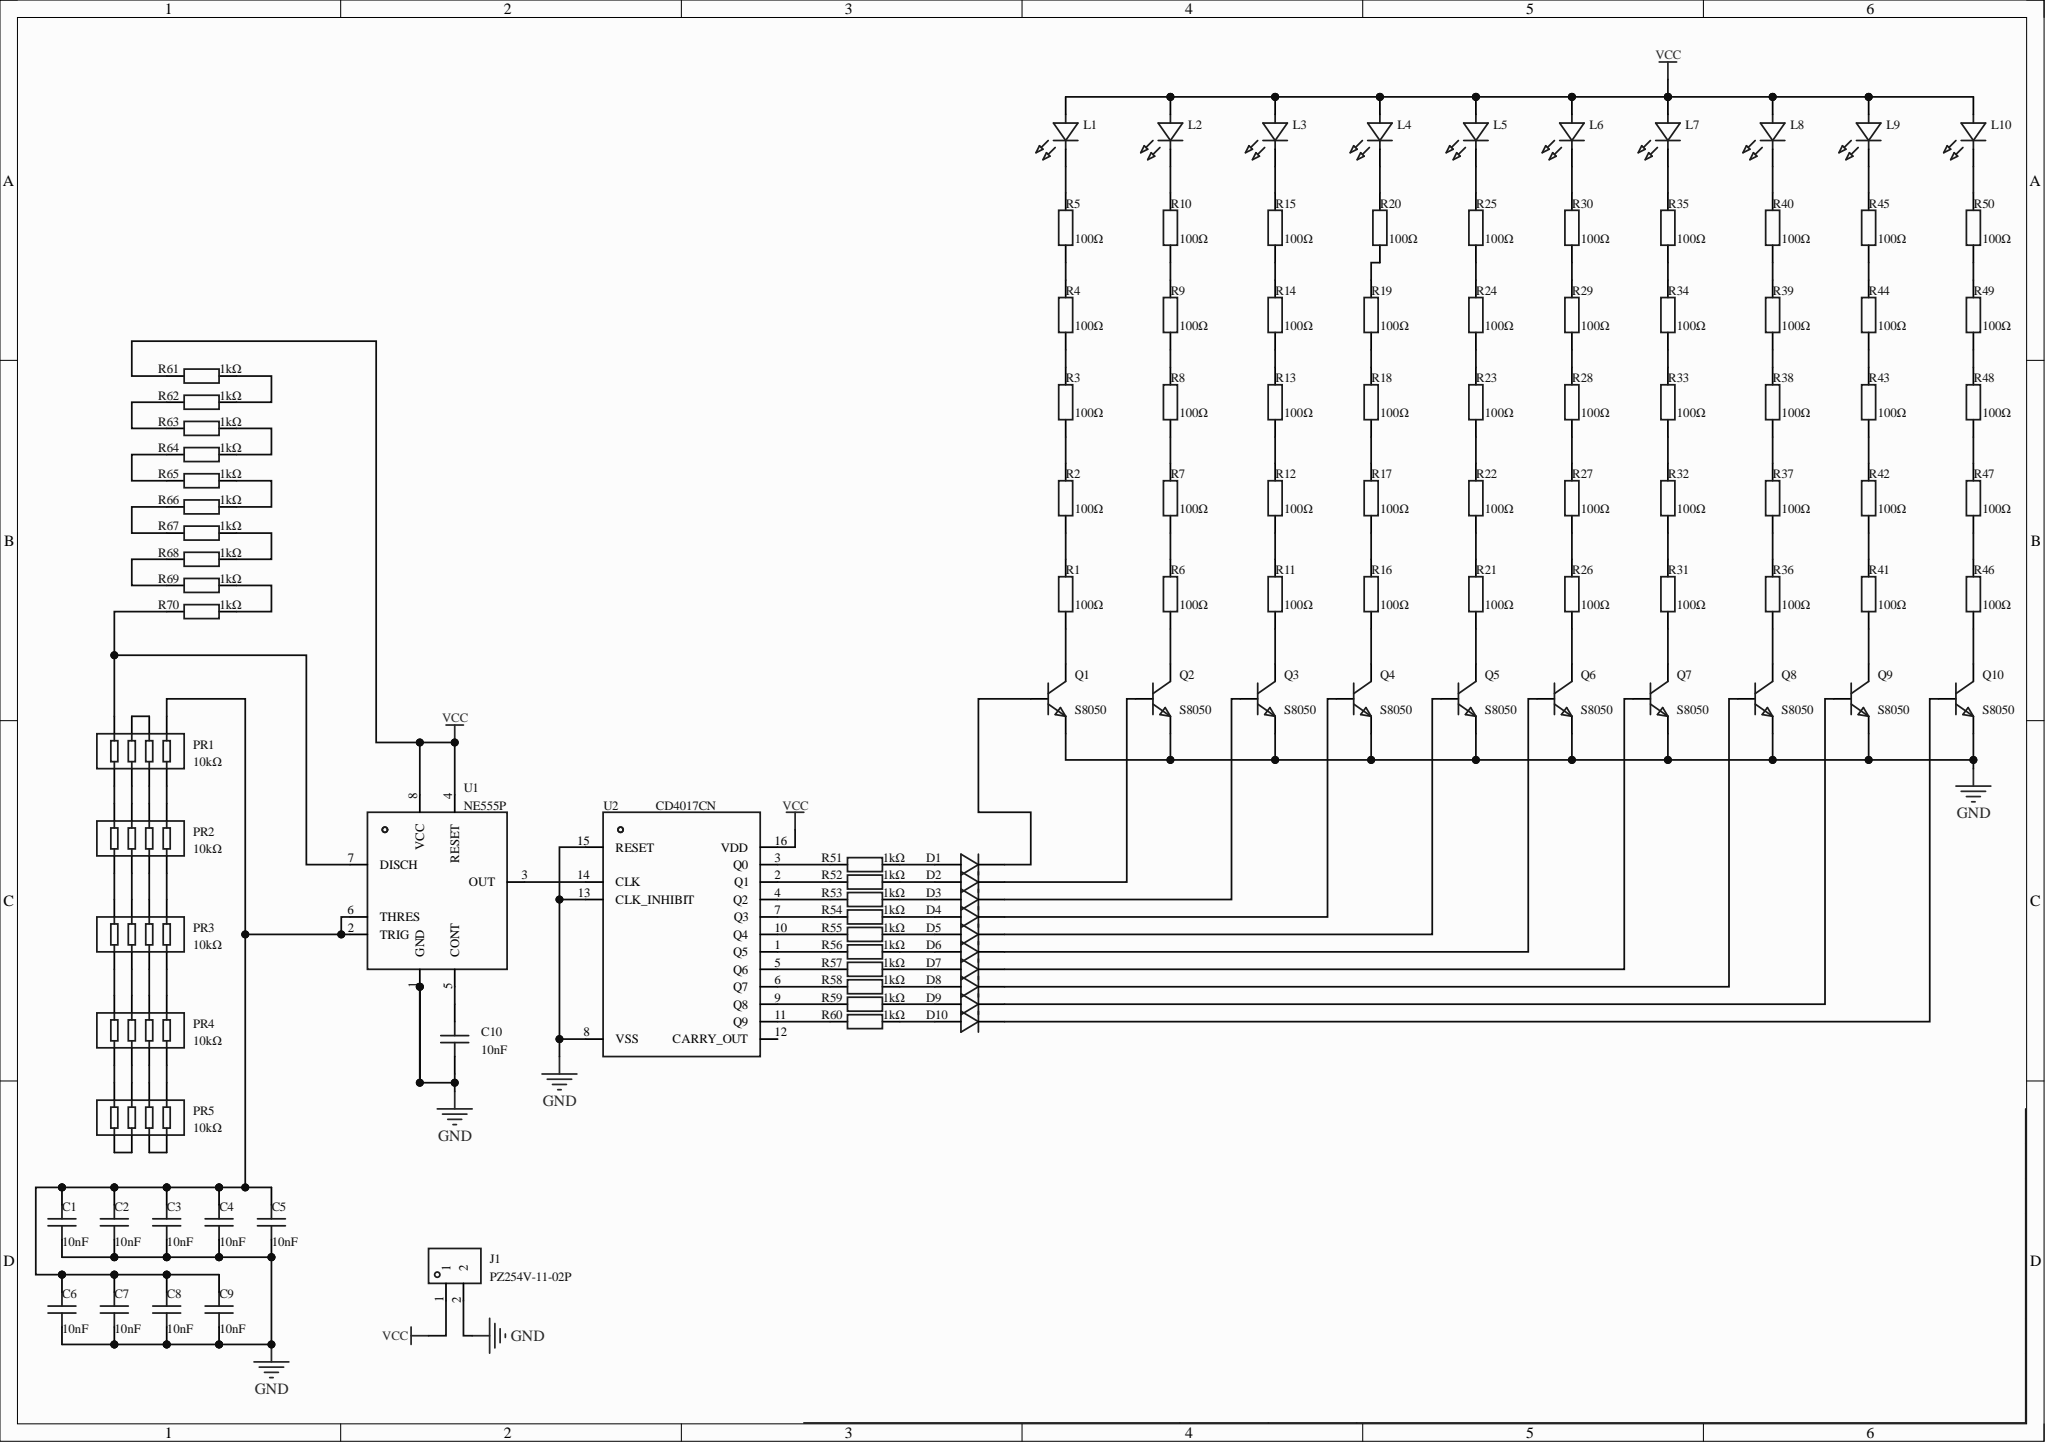Circuit board | Altium Designer | 118 parts | 124 nets
Bill of materials:
Comment,Description,Designator,Footprint,LibRef,Quantity
"10nF","容值:10nF;精度:±20%;额定电压:1kV;温度系数:Y5V;","C1, C2, C3, C4, C5, C6, C7, C8, C9, C10","CAP-TH_L8.0-W2.8-P5.08-D0.6","CC3A103MC1IEF48C30MF","10"
"1N4148TR","二极管配置:-;正向压降(Vf):1V@10mA;直流反向耐压(Vr):100V;整流电流:200mA;反向恢复时间(Trr):4ns;","D1, D2, D3, D4, D5, D6, D7, D8, D9, D10","DO-35_BD2.0-L4.2-P8.20-D0.5-RD","1N4148TR_C84410","10"
"PZ254V-11-02P","插针结构:1x2P;间距:2.54mm;行距:-;圆针/方针:方针;安装方式:直插;排数:单排;总PIN位数:2P;额定电流:3A;额定电压:250V;配合针长度:6mm;塑高:2.5mm;端接针长度:3mm;触头材质:黄铜;触头镀层:-;工作温度:-40℃~+105℃;颜色:黑色;","J1","HDR-TH_2P-P2.54-V-M","PZ254V-11-02P","1"
"XL-502SURD","灯头类型:5mm圆形灯头;发光颜色:红色;正向压降(Vf):2.4V;功率:70mW;正向电流:20mA;波长:615nm~625nm;二极管配置:-;透镜颜色:红色透镜;色温:-;发光强度:300mcd;发光角度:35°;载带方式:-;工作温度:-25℃~+85℃;","L1, L2, L3, L4, L5, L6, L7, L8, L9, L10","LED-TH_BD5.9-P2.54-RD_RED","XL-502SURD","10"
"10kΩ","","PR1, PR2, PR3, PR4, PR5","RES-ARRAY-TH_8P-L20.3-W2.5-P2.54","4608X-102-103LF","5"
"S8050","晶体管类型:NPN;集电极电流(Ic):500mA;集射极击穿电压(Vceo):25V;耗散功率(Pd):625mW;直流电流增益(hFE):160@50mA,1V;","Q1, Q2, Q3, Q4, Q5, Q6, Q7, Q8, Q9, Q10","TO-92-3_L4.5-W3.5-P1.27-L","S8050_C2931492","10"
"100Ω","","R1, R2, R3, R4, R5, R6, R7, R8, R9, R10, R11, R12, R13, R14, R15, R16, R17, R18, R19, R20, R21, R22, R23, R24, R25, R26, R27, R28, R29, R30, R31, R32, R33, R34, R35, R36, R37, R38, R39, R40, R41, R42, R43, R44, R45, R46, R47, R48, R49, R50","RES-TH_BD2.2-L6.5-P10.50-D0.6","MFR0W4F1000A50","50"
"1kΩ","","R51, R52, R53, R54, R55, R56, R57, R58, R59, R60, R61, R62, R63, R64, R65, R66, R67, R68, R69, R70","RES-TH_BD2.5-L6.5-P10.50-D0.6","MFR0W4F1001A50","20"
"NE555P","这些器件是精密定时电路，能够产生精确的时间延迟或振荡。在延时或单稳态工作模式下，定时时间间隔由单个外部电阻和电容网络控制。在无稳态工作模式下，频率和占空比可通过两个外部电阻和一个外部电容分别控制","U1","DIP-8_L9.8-W6.6-P2.54-LS7.6-BL","NE555P","1"
"CD4017CN","CD4017BE升级替代料，建议试样，5 阶 Johnson 译码计数器","U2","PDIP-16_L19.3-W6.4-P2.54-LS7.94-BL","CD4017CN","1"
Netlist (Protel format):
[
C1
CAP-TH_L8.0-W2.8-P5.08-D0.6
10nF



]
[
C2
CAP-TH_L8.0-W2.8-P5.08-D0.6
10nF



]
[
C3
CAP-TH_L8.0-W2.8-P5.08-D0.6
10nF



]
[
C4
CAP-TH_L8.0-W2.8-P5.08-D0.6
10nF



]
[
C5
CAP-TH_L8.0-W2.8-P5.08-D0.6
10nF



]
[
C6
CAP-TH_L8.0-W2.8-P5.08-D0.6
10nF



]
[
C7
CAP-TH_L8.0-W2.8-P5.08-D0.6
10nF



]
[
C8
CAP-TH_L8.0-W2.8-P5.08-D0.6
10nF



]
[
C9
CAP-TH_L8.0-W2.8-P5.08-D0.6
10nF



]
[
C10
CAP-TH_L8.0-W2.8-P5.08-D0.6
10nF



]
[
D1
DO-35_BD2.0-L4.2-P8.20-D0.5-RD
1N4148TR



]
[
D2
DO-35_BD2.0-L4.2-P8.20-D0.5-RD
1N4148TR



]
[
D3
DO-35_BD2.0-L4.2-P8.20-D0.5-RD
1N4148TR



]
[
D4
DO-35_BD2.0-L4.2-P8.20-D0.5-RD
1N4148TR



]
[
D5
DO-35_BD2.0-L4.2-P8.20-D0.5-RD
1N4148TR



]
[
D6
DO-35_BD2.0-L4.2-P8.20-D0.5-RD
1N4148TR



]
[
D7
DO-35_BD2.0-L4.2-P8.20-D0.5-RD
1N4148TR



]
[
D8
DO-35_BD2.0-L4.2-P8.20-D0.5-RD
1N4148TR



]
[
D9
DO-35_BD2.0-L4.2-P8.20-D0.5-RD
1N4148TR



]
[
D10
DO-35_BD2.0-L4.2-P8.20-D0.5-RD
1N4148TR



]
[
J1
HDR-TH_2P-P2.54-V-M
PZ254V-11-02P



]
[
L1
LED-TH_BD5.9-P2.54-RD_RED
XL-502SURD



]
[
L2
LED-TH_BD5.9-P2.54-RD_RED
XL-502SURD



]
[
L3
LED-TH_BD5.9-P2.54-RD_RED
XL-502SURD



]
[
L4
LED-TH_BD5.9-P2.54-RD_RED
XL-502SURD



]
[
L5
LED-TH_BD5.9-P2.54-RD_RED
XL-502SURD



]
[
L6
LED-TH_BD5.9-P2.54-RD_RED
XL-502SURD



]
[
L7
LED-TH_BD5.9-P2.54-RD_RED
XL-502SURD



]
[
L8
LED-TH_BD5.9-P2.54-RD_RED
XL-502SURD



]
[
L9
LED-TH_BD5.9-P2.54-RD_RED
XL-502SURD



]
[
L10
LED-TH_BD5.9-P2.54-RD_RED
XL-502SURD



]
[
PR1
RES-ARRAY-TH_8P-L20.3-W2.5-P2.54
10kΩ



]
[
PR2
RES-ARRAY-TH_8P-L20.3-W2.5-P2.54
10kΩ



]
[
PR3
RES-ARRAY-TH_8P-L20.3-W2.5-P2.54
10kΩ



]
[
PR4
RES-ARRAY-TH_8P-L20.3-W2.5-P2.54
10kΩ



]
[
PR5
RES-ARRAY-TH_8P-L20.3-W2.5-P2.54
10kΩ



]
[
Q1
TO-92-3_L4.5-W3.5-P1.27-L
S8050



]
[
Q2
TO-92-3_L4.5-W3.5-P1.27-L
S8050



]
[
Q3
TO-92-3_L4.5-W3.5-P1.27-L
S8050



]
[
Q4
TO-92-3_L4.5-W3.5-P1.27-L
S8050



]
[
Q5
TO-92-3_L4.5-W3.5-P1.27-L
S8050



]
[
Q6
TO-92-3_L4.5-W3.5-P1.27-L
S8050



]
[
Q7
TO-92-3_L4.5-W3.5-P1.27-L
S8050



]
[
Q8
TO-92-3_L4.5-W3.5-P1.27-L
S8050



]
[
Q9
TO-92-3_L4.5-W3.5-P1.27-L
S8050



]
[
Q10
TO-92-3_L4.5-W3.5-P1.27-L
S8050



]
[
R1
RES-TH_BD2.2-L6.5-P10.50-D0.6
100Ω



]
[
R2
RES-TH_BD2.2-L6.5-P10.50-D0.6
100Ω



]
[
R3
RES-TH_BD2.2-L6.5-P10.50-D0.6
100Ω



]
[
R4
RES-TH_BD2.2-L6.5-P10.50-D0.6
100Ω



]
[
R5
RES-TH_BD2.2-L6.5-P10.50-D0.6
100Ω



]
[
R6
RES-TH_BD2.2-L6.5-P10.50-D0.6
100Ω



]
[
R7
RES-TH_BD2.2-L6.5-P10.50-D0.6
100Ω



]
[
R8
RES-TH_BD2.2-L6.5-P10.50-D0.6
100Ω



]
[
R9
RES-TH_BD2.2-L6.5-P10.50-D0.6
100Ω



]
[
R10
RES-TH_BD2.2-L6.5-P10.50-D0.6
100Ω



]
[
R11
RES-TH_BD2.2-L6.5-P10.50-D0.6
100Ω



]
[
R12
RES-TH_BD2.2-L6.5-P10.50-D0.6
100Ω



]
[
R13
RES-TH_BD2.2-L6.5-P10.50-D0.6
100Ω



]
[
R14
RES-TH_BD2.2-L6.5-P10.50-D0.6
100Ω



]
[
R15
RES-TH_BD2.2-L6.5-P10.50-D0.6
100Ω



]
[
R16
RES-TH_BD2.2-L6.5-P10.50-D0.6
100Ω



]
[
R17
RES-TH_BD2.2-L6.5-P10.50-D0.6
100Ω



]
[
R18
RES-TH_BD2.2-L6.5-P10.50-D0.6
100Ω



]
[
R19
RES-TH_BD2.2-L6.5-P10.50-D0.6
100Ω



]
[
R20
RES-TH_BD2.2-L6.5-P10.50-D0.6
100Ω



]
[
R21
RES-TH_BD2.2-L6.5-P10.50-D0.6
100Ω



]
[
R22
RES-TH_BD2.2-L6.5-P10.50-D0.6
100Ω



]
[
R23
RES-TH_BD2.2-L6.5-P10.50-D0.6
100Ω



]
[
R24
RES-TH_BD2.2-L6.5-P10.50-D0.6
100Ω



]
[
R25
RES-TH_BD2.2-L6.5-P10.50-D0.6
100Ω



]
[
R26
RES-TH_BD2.2-L6.5-P10.50-D0.6
100Ω



]
[
R27
RES-TH_BD2.2-L6.5-P10.50-D0.6
100Ω



]
[
R28
RES-TH_BD2.2-L6.5-P10.50-D0.6
100Ω



]
[
R29
RES-TH_BD2.2-L6.5-P10.50-D0.6
100Ω



]
[
R30
RES-TH_BD2.2-L6.5-P10.50-D0.6
100Ω



]
[
R31
RES-TH_BD2.2-L6.5-P10.50-D0.6
100Ω



]
[
R32
RES-TH_BD2.2-L6.5-P10.50-D0.6
100Ω



]
[
R33
RES-TH_BD2.2-L6.5-P10.50-D0.6
100Ω



]
[
R34
RES-TH_BD2.2-L6.5-P10.50-D0.6
100Ω



]
[
R35
RES-TH_BD2.2-L6.5-P10.50-D0.6
100Ω



]
[
R36
RES-TH_BD2.2-L6.5-P10.50-D0.6
100Ω



]
[
R37
RES-TH_BD2.2-L6.5-P10.50-D0.6
100Ω



]
[
R38
RES-TH_BD2.2-L6.5-P10.50-D0.6
100Ω



]
[
R39
RES-TH_BD2.2-L6.5-P10.50-D0.6
100Ω



]
[
R40
RES-TH_BD2.2-L6.5-P10.50-D0.6
100Ω



]
[
R41
RES-TH_BD2.2-L6.5-P10.50-D0.6
100Ω



]
[
R42
RES-TH_BD2.2-L6.5-P10.50-D0.6
100Ω



]
[
R43
RES-TH_BD2.2-L6.5-P10.50-D0.6
100Ω



]
[
R44
RES-TH_BD2.2-L6.5-P10.50-D0.6
100Ω



]
[
R45
RES-TH_BD2.2-L6.5-P10.50-D0.6
100Ω



]
[
R46
RES-TH_BD2.2-L6.5-P10.50-D0.6
100Ω



]
[
R47
RES-TH_BD2.2-L6.5-P10.50-D0.6
100Ω



]
[
R48
RES-TH_BD2.2-L6.5-P10.50-D0.6
100Ω



]
[
R49
RES-TH_BD2.2-L6.5-P10.50-D0.6
100Ω



]
[
R50
RES-TH_BD2.2-L6.5-P10.50-D0.6
100Ω



]
[
R51
RES-TH_BD2.5-L6.5-P10.50-D0.6
1kΩ



]
[
R52
RES-TH_BD2.5-L6.5-P10.50-D0.6
1kΩ



]
[
R53
RES-TH_BD2.5-L6.5-P10.50-D0.6
1kΩ



]
[
R54
RES-TH_BD2.5-L6.5-P10.50-D0.6
1kΩ



]
[
R55
RES-TH_BD2.5-L6.5-P10.50-D0.6
1kΩ



]
[
R56
RES-TH_BD2.5-L6.5-P10.50-D0.6
1kΩ



]
[
R57
RES-TH_BD2.5-L6.5-P10.50-D0.6
1kΩ



]
[
R58
RES-TH_BD2.5-L6.5-P10.50-D0.6
1kΩ



]
[
R59
RES-TH_BD2.5-L6.5-P10.50-D0.6
1kΩ



]
[
R60
RES-TH_BD2.5-L6.5-P10.50-D0.6
1kΩ



]
[
R61
RES-TH_BD2.5-L6.5-P10.50-D0.6
1kΩ



]
[
R62
RES-TH_BD2.5-L6.5-P10.50-D0.6
1kΩ



]
[
R63
RES-TH_BD2.5-L6.5-P10.50-D0.6
1kΩ



]
[
R64
RES-TH_BD2.5-L6.5-P10.50-D0.6
1kΩ



]
[
R65
RES-TH_BD2.5-L6.5-P10.50-D0.6
1kΩ



]
[
R66
RES-TH_BD2.5-L6.5-P10.50-D0.6
1kΩ



]
[
R67
RES-TH_BD2.5-L6.5-P10.50-D0.6
1kΩ



]
[
R68
RES-TH_BD2.5-L6.5-P10.50-D0.6
1kΩ



]
[
R69
RES-TH_BD2.5-L6.5-P10.50-D0.6
1kΩ



]
[
R70
RES-TH_BD2.5-L6.5-P10.50-D0.6
1kΩ



]
[
U1
DIP-8_L9.8-W6.6-P2.54-LS7.6-BL
NE555P



]
[
U2
PDIP-16_L19.3-W6.4-P2.54-LS7.94-BL
CD4017CN



]
(
VCC
J1-1
L1-2
L2-2
L3-2
L4-2
L5-2
L6-2
L7-2
L8-2
L9-2
L10-2
R61-1
U1-4
U1-8
U2-16
)
(
NetU1_3
U1-3
U2-14
)
(
NetR69_2
R69-2
R70-2
)
(
NetR68_1
R68-1
R69-1
)
(
NetR67_2
R67-2
R68-2
)
(
NetR66_1
R66-1
R67-1
)
(
NetR65_2
R65-2
R66-2
)
(
NetR64_1
R64-1
R65-1
)
(
NetR63_2
R63-2
R64-2
)
(
NetR62_1
R62-1
R63-1
)
(
NetR61_2
R61-2
R62-2
)
(
NetR60_1
R60-1
U2-11
)
(
NetR59_1
R59-1
U2-9
)
(
NetR58_1
R58-1
U2-6
)
(
NetR57_1
R57-1
U2-5
)
(
NetR56_1
R56-1
U2-1
)
(
NetR55_1
R55-1
U2-10
)
(
NetR54_1
R54-1
U2-7
)
(
NetR53_1
R53-1
U2-4
)
(
NetR52_1
R52-1
U2-2
)
(
NetR51_1
R51-1
U2-3
)
(
NetR49_2
R49-2
R50-1
)
(
NetR48_2
R48-2
R49-1
)
(
NetR47_2
R47-2
R48-1
)
(
NetR46_2
R46-2
R47-1
)
(
NetR44_2
R44-2
R45-1
)
(
NetR43_2
R43-2
R44-1
)
(
NetR42_2
R42-2
R43-1
)
(
NetR41_2
R41-2
R42-1
)
(
NetR39_2
R39-2
R40-1
)
(
NetR38_2
R38-2
R39-1
)
(
NetR37_2
R37-2
R38-1
)
(
NetR36_2
R36-2
R37-1
)
(
NetR34_2
R34-2
R35-1
)
(
NetR33_2
R33-2
R34-1
)
(
NetR32_2
R32-2
R33-1
)
(
NetR31_2
R31-2
R32-1
)
(
NetR29_2
R29-2
R30-1
)
(
NetR28_2
R28-2
R29-1
)
(
NetR27_2
R27-2
R28-1
)
(
NetR26_2
R26-2
R27-1
)
(
NetR24_2
R24-2
R25-1
)
(
NetR23_2
R23-2
R24-1
)
(
NetR22_2
R22-2
R23-1
)
(
NetR21_2
R21-2
R22-1
)
(
NetR19_2
R19-2
R20-1
)
(
NetR18_2
R18-2
R19-1
)
(
NetR17_2
R17-2
R18-1
)
(
NetR16_2
R16-2
R17-1
)
(
NetR14_2
R14-2
R15-1
)
(
NetR13_2
R13-2
R14-1
)
(
NetR12_2
R12-2
R13-1
)
(
NetR11_2
R11-2
R12-1
)
(
NetR9_2
R9-2
R10-1
)
(
NetR8_2
R8-2
R9-1
)
(
NetR7_2
R7-2
R8-1
)
(
NetR6_2
R6-2
R7-1
)
(
NetR4_2
R4-2
R5-1
)
(
NetR3_2
R3-2
R4-1
)
(
NetR2_2
R2-2
R3-1
)
(
NetR1_2
R1-2
R2-1
)
(
NetQ10_3
Q10-3
R46-1
)
(
NetQ9_3
Q9-3
R41-1
)
(
NetQ8_3
Q8-3
R36-1
)
(
NetQ7_3
Q7-3
R31-1
)
(
NetQ6_3
Q6-3
R26-1
)
(
NetQ5_3
Q5-3
R21-1
)
(
NetQ4_3
Q4-3
R16-1
)
(
NetQ3_3
Q3-3
R11-1
)
(
NetQ2_3
Q2-3
R6-1
)
(
NetQ1_3
Q1-3
R1-1
)
(
NetPR5_3
PR5-3
PR5-4
)
(
NetPR5_1
PR5-1
PR5-2
)
(
NetPR4_4
PR4-4
PR5-5
)
(
NetPR4_3
PR4-3
PR5-6
)
(
NetPR4_2
PR4-2
PR5-7
)
(
NetPR4_1
PR4-1
PR5-8
)
(
NetPR3_4
PR3-4
PR4-5
)
(
NetPR3_3
PR3-3
PR4-6
)
(
NetPR3_2
PR3-2
PR4-7
)
(
NetPR3_1
PR3-1
PR4-8
)
(
NetPR2_4
PR2-4
PR3-5
)
(
NetPR2_3
PR2-3
PR3-6
)
(
NetPR2_2
PR2-2
PR3-7
)
(
NetPR2_1
PR2-1
PR3-8
)
(
NetPR1_8
PR1-8
R70-1
U1-7
)
(
NetPR1_6
PR1-6
PR1-7
)
(
NetPR1_4
PR1-4
PR2-5
)
(
NetPR1_3
PR1-3
PR2-6
)
(
NetPR1_2
PR1-2
PR2-7
)
(
NetPR1_1
PR1-1
PR2-8
)
(
NetL10_1
L10-1
R50-2
)
(
NetL9_1
L9-1
R45-2
)
(
NetL8_1
L8-1
R40-2
)
(
NetL7_1
L7-1
R35-2
)
(
NetL6_1
L6-1
R30-2
)
(
NetL5_1
L5-1
R25-2
)
(
NetL4_1
L4-1
R20-2
)
(
NetL3_1
L3-1
R15-2
)
(
NetL2_1
L2-1
R10-2
)
(
NetL1_1
L1-1
R5-2
)
(
NetD10_2
D10-2
R60-2
)
(
NetD10_1
D10-1
Q10-2
)
(
NetD9_2
D9-2
R59-2
)
(
NetD9_1
D9-1
Q9-2
)
(
NetD8_2
D8-2
R58-2
)
(
NetD8_1
D8-1
Q8-2
)
(
NetD7_2
D7-2
R57-2
)
(
NetD7_1
D7-1
Q7-2
)
(
NetD6_2
D6-2
R56-2
)
(
NetD6_1
D6-1
Q6-2
)
(
NetD5_2
D5-2
R55-2
)
(
NetD5_1
D5-1
Q5-2
)
(
NetD4_2
D4-2
R54-2
)
(
NetD4_1
D4-1
Q4-2
)
(
NetD3_2
D3-2
R53-2
)
(
NetD3_1
D3-1
Q3-2
)
(
NetD2_2
D2-2
R52-2
)
(
NetD2_1
D2-1
Q2-2
)
(
NetD1_2
D1-2
R51-2
)
(
NetD1_1
D1-1
Q1-2
)
(
NetC10_2
C10-2
U1-5
)
(
NetC1_2
C1-2
C2-2
C3-2
C4-2
C5-2
C6-2
C7-2
C8-2
C9-2
PR1-5
U1-2
U1-6
)
(
GND
C1-1
C2-1
C3-1
C4-1
C5-1
C6-1
C7-1
C8-1
C9-1
C10-1
J1-2
Q1-1
Q2-1
Q3-1
Q4-1
Q5-1
Q6-1
Q7-1
Q8-1
Q9-1
Q10-1
U1-1
U2-8
U2-13
U2-15
)